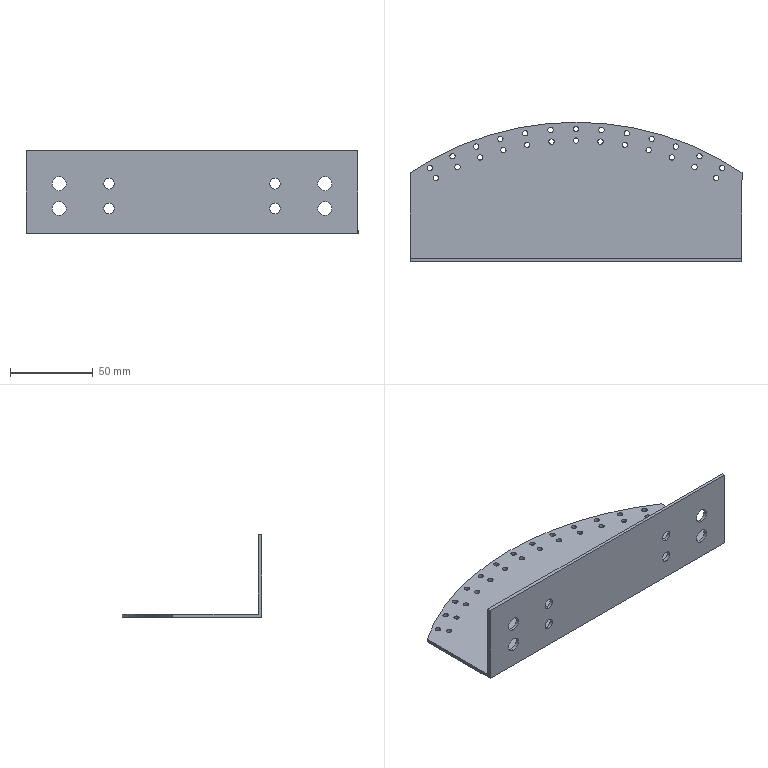Part | SolidWorks | features ICE 2, Extrusion 1 | 1 solid | 76 faces | box 200 x 84 x 50 mm | volume 47784 mm3 | cylinder 69 | plane 7 | commonest cylinder face diameters 3.2 x52 6.4 x8 8.4 x8 360 x1